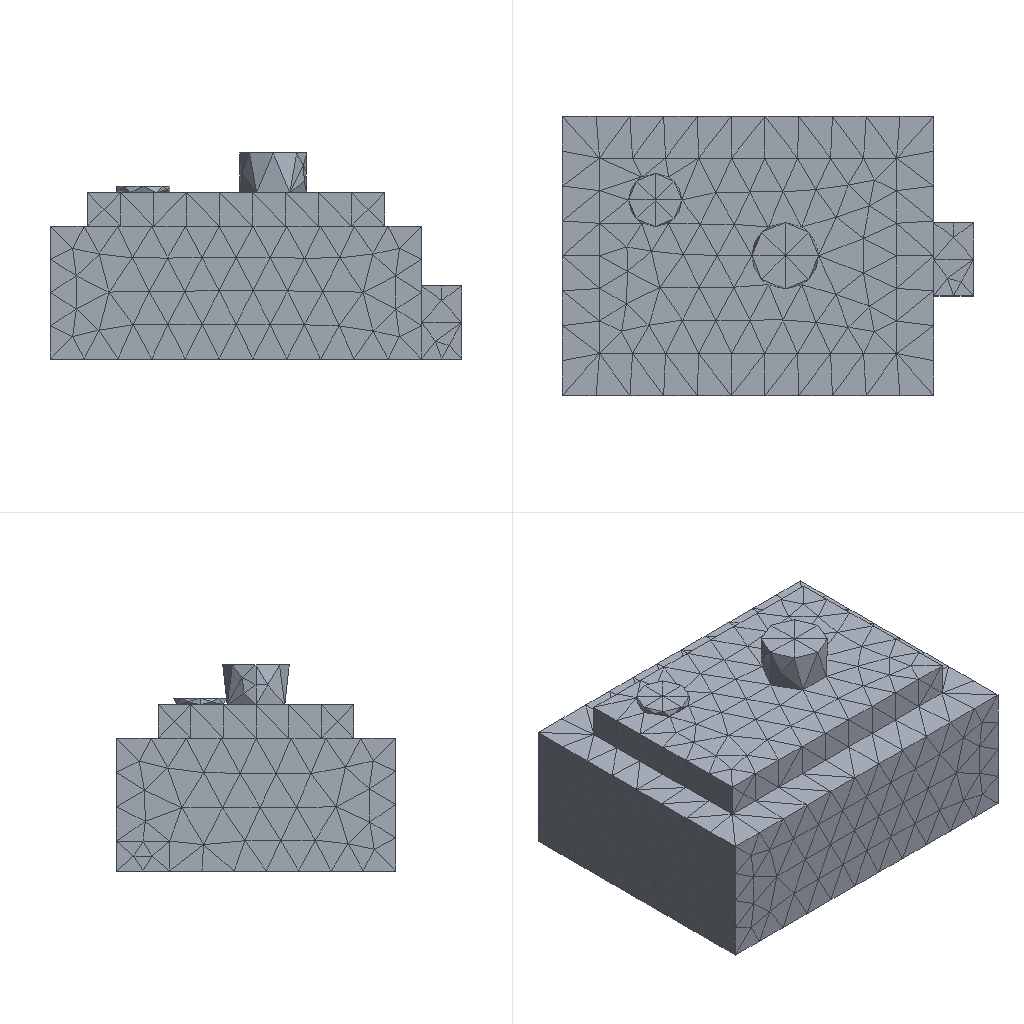Simulation study | ansys mapdl
Set-up summary:
category,name,step,type,value,unit,region
solver,ansys_mapdl
units,mm-N-s-tonne (MPa),,inferred,E=210000 density=
analysis,model,,static
mesh,nodes,,,5555
mesh,elements,,,3409
element_type,SOLID187,,,3409
material,mat 1,,E,210000
material,mat 1,,nu,0.3
load,,model,body load temp,,,all
load,,model,force,"1000 [dir=(0, 0, -1) n=186]",,node list
bc,,model,fixed,"[dofs=UX,UY,UZ n=5758]",,node list
Ansys APDL input file, long lists of numbers shortened:
/COM,ANSYS RELEASE 2026 R1           BUILD 26.1      UP20260202       09:10:51
/PREP7
/NOPR
/TITLE,2
ANTYPE, 0
*IF,_CDRDOFF,EQ,1,THEN     !if solid model was read in
_CDRDOFF=             !reset flag, numoffs already performed
*ELSE              !offset database for the following FE model
NUMOFF,NODE,     5555
NUMOFF,ELEM,     3409
NUMOFF,MAT ,        1
NUMOFF,TYPE,        1
*ENDIF
*SET,_RETURN ,  0.
*SET,_STATUS ,  0.
*SET,_UIQR   ,  186.
*SET,__FLOATPARAMETER__,  5555.
DOF,DELETE
ETBLOCK,        1,        1
(2i9,19a9)
        1      187        0        0        0        0        0        0        0        0        0        0        0        0        0        0        0        0        0        0        0
       -1
NBLOCK,6,SOLID,      5555,      5555
(3i9,6e21.13e3)
        1        0        0-3.9850000000000E+001 4.2000000000000E+001 9.0000000000000E+000
! (5554 more lines like these left out)
N,UNBL,LOC,       -1,
EBLOCK,19,SOLID,      3409,      3409
(19i10)
         1         1         1         1         0         0         0         0        10         0         1      1919      1920      1921      1922      2272      2273      2274      2275
! (6817 more lines like these left out)
        -1
MPTEMP,UNBL, 1, 1,  0.    ,
MPDATA,UNBL, 1,EX  ,       1, 1,  210000.000    ,
MPTEMP,UNBL, 1, 1,  0.    ,
MPDATA,UNBL, 1,NUXY,       1, 1, 0.3    ,
MPTEMP,UNBL, 1, 1,  0.    ,
MPDATA,UNBL, 1,PRXY,       1, 1, 0.3    ,
EXTOPT,ATTR,      0,      0,      0
EXTOPT,ESIZE,  0,  0.
EXTOPT,ACLEAR,      0
TREF,  0.
IRLF,  0
BFUNIF,TEMP,_TINY
ACEL,  0.    ,  0.    ,  0.
OMEGA,  0.    ,  0.    ,  0.
DOMEGA,  0.    ,  0.    ,  0.
CGLOC,  0.    ,  0.    ,  0.
CGOMEGA,  0.    ,  0.    ,  0.
DCGOMG,  0.    ,  0.    ,  0.
KUSE,     0
TIME,  0.
ALPHAD,  0.
BETAD,  0.
DMPRAT,  0.
DMPSTR,  0.
CRPLIM, 0.1    ,   0
CRPLIM,  0.    ,   1
NCNV,     0, 1.000000000E+12,     0,  0.    ,  0.
NEQIT,     0
ERESX,DEFA
DBLOCK,      5758
(i9,a6,2(pg16.9))
        1  UX    0.00000000      0.00000000
! (5757 more lines like these left out)
       -1
FBLOCK,       186
(i9,a6,2(pg16.9))
      912  FZ   -5.37634409      0.00000000
! (185 more lines like these left out)
       -1
/GO
FINISH
Results summary:
result,analysis_type_db,,,static,unstated
result,n_sets,,,1,unstated
result,load_steps[0].set,load_step=1,,1,unstated
result,load_steps[0].substep,load_step=1,,1,unstated
result,load_steps[0].time,load_step=1,,1,unstated
result,load_steps[0].freq,load_step=1,,1,unstated
result,load_steps[0].max_usum,load_step=1,,0.0002522,unstated
result,load_steps[0].max_seqv,load_step=1,,3.228,unstated
result,load_steps[0].reaction_sum.FX,load_step=1,,-2.85256e-11,unstated
result,load_steps[0].reaction_sum.FY,load_step=1,,3.29692e-12,unstated
result,load_steps[0].reaction_sum.FZ,load_step=1,,1000,unstated
result,load_steps[0].reaction_sum.MX,load_step=1,,0,unstated
result,load_steps[0].reaction_sum.MY,load_step=1,,0,unstated
result,load_steps[0].reaction_sum.MZ,load_step=1,,0,unstated
result,convergence,,,results present for all listed sets,unstated